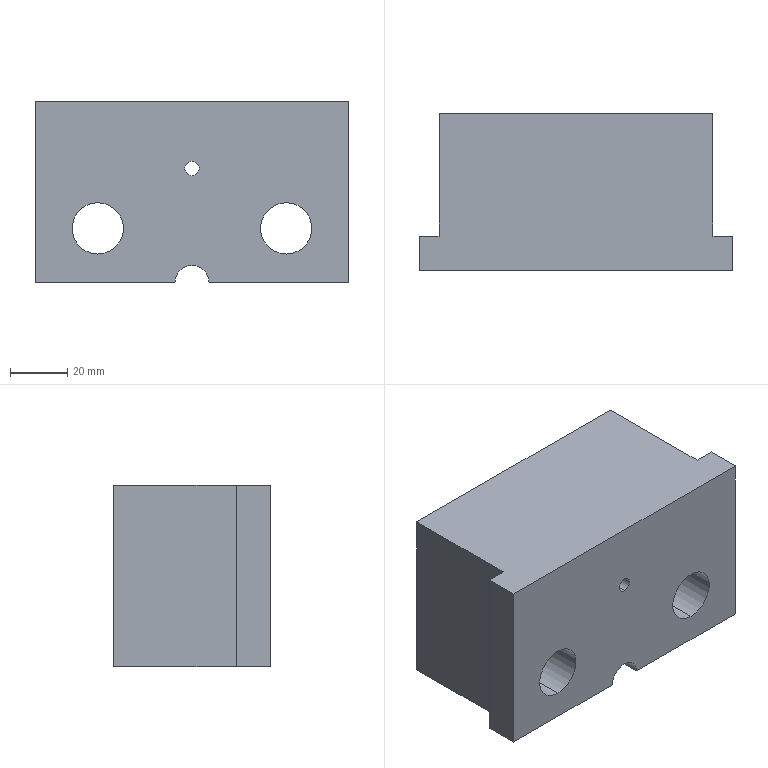Part | STEP file | 001-009-Riveting mechanism lower die spacer block | 1 solid | 29 faces | box 110 x 55 x 63.5 mm | volume 312289 mm3 | plane 13 | cylinder 12 | cone 4 | commonest cylinder face diameters 18 x4 25 x4 5 x2 12 x2